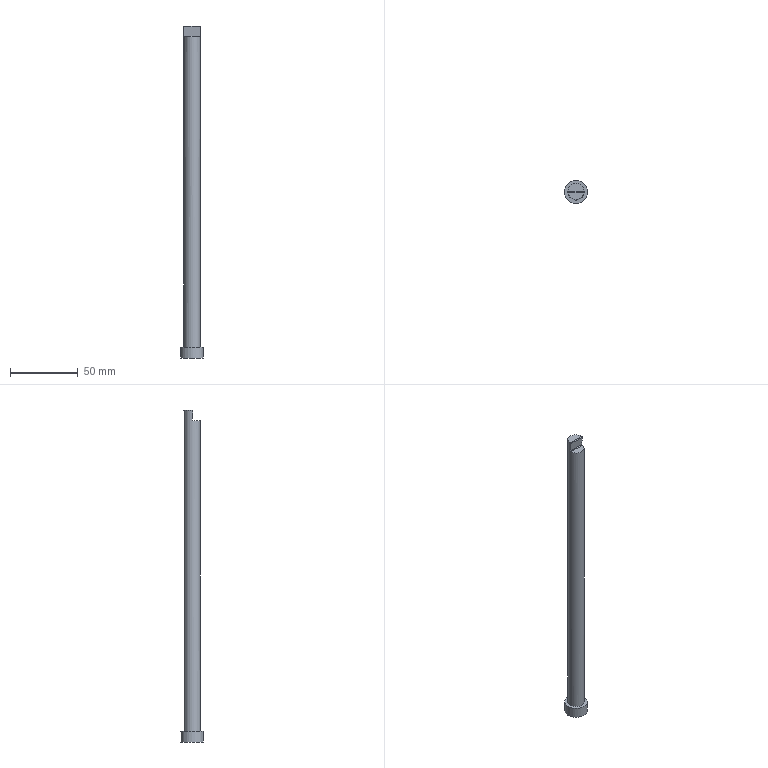Part | NX | features 模具.stp<1>[104] 2 | 1 solid | 9 faces | box 17 x 17 x 245.5 mm | volume 28258 mm3 | plane 5 | cylinder 4 | commonest cylinder face diameters 1 x2 12 x1 17 x1
STEP:
#1=CARTESIAN_POINT('',(-5.998,-0.1543,30.));
#2=VERTEX_POINT('',#1);
#3=CARTESIAN_POINT('',(-5.964,-0.6524,29.456));
#4=VERTEX_POINT('',#3);
#5=CARTESIAN_POINT('',(-5.998,-0.1543,30.));
#6=CARTESIAN_POINT('',(-5.992,-0.406,30.));
#7=CARTESIAN_POINT('',(-5.962,-0.6742,29.706));
#8=CARTESIAN_POINT('',(-5.964,-0.6524,29.456));
#9=B_SPLINE_CURVE_WITH_KNOTS('',3,(#5,#6,#7,#8),.UNSPECIFIED.,.F.,.F.,(4,4),(0.,1.),.UNSPECIFIED.);
#10=EDGE_CURVE('',#2,#4,#9,.T.);
#11=ORIENTED_EDGE('',*,*,#10,.T.);
#12=CARTESIAN_POINT('',(5.964,-0.6524,29.456));
#13=VERTEX_POINT('',#12);
#14=CARTESIAN_POINT('',(6.,-0.6524,29.456));
#15=DIRECTION('',(-1.,0.,0.));
#16=VECTOR('',#15,1000.);
#17=LINE('',#14,#16);
#18=EDGE_CURVE('',#13,#4,#17,.T.);
#19=ORIENTED_EDGE('',*,*,#18,.F.);
#20=CARTESIAN_POINT('',(5.998,-0.1543,30.));
#21=VERTEX_POINT('',#20);
#22=CARTESIAN_POINT('',(5.964,-0.6524,29.456));
#23=CARTESIAN_POINT('',(5.962,-0.6723,29.684));
#24=CARTESIAN_POINT('',(5.99,-0.4503,30.));
#25=CARTESIAN_POINT('',(5.998,-0.1543,30.));
#26=B_SPLINE_CURVE_WITH_KNOTS('',3,(#22,#23,#24,#25),.UNSPECIFIED.,.F.,.F.,(4,4),(0.,1.),.UNSPECIFIED.);
#27=EDGE_CURVE('',#13,#21,#26,.T.);
#28=ORIENTED_EDGE('',*,*,#27,.T.);
#29=CARTESIAN_POINT('',(0.,-0.1543,30.));
#30=DIRECTION('',(-1.,0.,0.));
#31=VECTOR('',#30,1000.);
#32=LINE('',#29,#31);
#33=EDGE_CURVE('',#21,#2,#32,.T.);
#34=ORIENTED_EDGE('',*,*,#33,.T.);
#35=EDGE_LOOP('',(#11,#19,#28,#34));
#36=FACE_BOUND('',#35,.T.);
#37=CARTESIAN_POINT('',(6.,-0.1543,29.5));
#38=DIRECTION('',(1.,0.,0.));
#39=DIRECTION('',(0.,0.,-1.));
#40=AXIS2_PLACEMENT_3D('',#37,#38,#39);
#41=CYLINDRICAL_SURFACE('',#40,0.5);
#42=ADVANCED_FACE('',(#36),#41,.T.);
#43=CARTESIAN_POINT('',(5.975,-0.5457,22.));
#44=VERTEX_POINT('',#43);
#45=CARTESIAN_POINT('',(6.,-0.04756,22.544));
#46=VERTEX_POINT('',#45);
#47=CARTESIAN_POINT('',(5.975,-0.5457,22.));
#48=CARTESIAN_POINT('',(5.987,-0.4152,22.));
#49=CARTESIAN_POINT('',(6.001,-0.1315,22.146));
#50=CARTESIAN_POINT('',(6.,-0.03109,22.355));
#51=CARTESIAN_POINT('',(6.,-0.04756,22.544));
#52=B_SPLINE_CURVE_WITH_KNOTS('',3,(#47,#48,#49,#50,#51),.UNSPECIFIED.,.F.,.F.,(4,1,4),(0.,0.5,1.),.UNSPECIFIED.);
#53=EDGE_CURVE('',#44,#46,#52,.T.);
#54=ORIENTED_EDGE('',*,*,#53,.T.);
#55=CARTESIAN_POINT('',(-6.,-0.04756,22.544));
#56=VERTEX_POINT('',#55);
#57=CARTESIAN_POINT('',(-6.,-0.04756,22.544));
#58=DIRECTION('',(1.,0.,0.));
#59=VECTOR('',#58,1000.);
#60=LINE('',#57,#59);
#61=EDGE_CURVE('',#56,#46,#60,.T.);
#62=ORIENTED_EDGE('',*,*,#61,.F.);
#63=CARTESIAN_POINT('',(-5.975,-0.5457,22.));
#64=VERTEX_POINT('',#63);
#65=CARTESIAN_POINT('',(-6.,-0.04756,22.544));
#66=CARTESIAN_POINT('',(-6.,-0.0311,22.355));
#67=CARTESIAN_POINT('',(-6.001,-0.1312,22.146));
#68=CARTESIAN_POINT('',(-5.987,-0.4151,22.));
#69=CARTESIAN_POINT('',(-5.975,-0.5457,22.));
#70=B_SPLINE_CURVE_WITH_KNOTS('',3,(#65,#66,#67,#68,#69),.UNSPECIFIED.,.F.,.F.,(4,1,4),(0.,0.5,1.),.UNSPECIFIED.);
#71=EDGE_CURVE('',#56,#64,#70,.T.);
#72=ORIENTED_EDGE('',*,*,#71,.T.);
#73=CARTESIAN_POINT('',(6.,-0.5457,22.));
#74=DIRECTION('',(-1.,0.,0.));
#75=VECTOR('',#74,1000.);
#76=LINE('',#73,#75);
#77=EDGE_CURVE('',#44,#64,#76,.T.);
#78=ORIENTED_EDGE('',*,*,#77,.F.);
#79=EDGE_LOOP('',(#54,#62,#72,#78));
#80=FACE_BOUND('',#79,.T.);
#81=CARTESIAN_POINT('',(6.,-0.5457,22.5));
#82=DIRECTION('',(1.,0.,0.));
#83=DIRECTION('',(0.,0.,-1.));
#84=AXIS2_PLACEMENT_3D('',#81,#82,#83);
#85=CYLINDRICAL_SURFACE('',#84,0.5);
#86=ADVANCED_FACE('',(#80),#85,.F.);
#87=CARTESIAN_POINT('',(0.,0.,22.));
#88=DIRECTION('',(0.,0.9962,0.08716));
#89=DIRECTION('',(0.,-0.08716,0.9962));
#90=AXIS2_PLACEMENT_3D('',#87,#88,#89);
#91=ELLIPSE('',#90,68.842,6.);
#92=EDGE_CURVE('',#13,#46,#91,.T.);
#93=ORIENTED_EDGE('',*,*,#92,.F.);
#94=ORIENTED_EDGE('',*,*,#18,.T.);
#95=CARTESIAN_POINT('',(0.,0.,22.));
#96=DIRECTION('',(0.,0.9962,0.08716));
#97=DIRECTION('',(0.,-0.08716,0.9962));
#98=AXIS2_PLACEMENT_3D('',#95,#96,#97);
#99=ELLIPSE('',#98,68.842,6.);
#100=EDGE_CURVE('',#56,#4,#99,.T.);
#101=ORIENTED_EDGE('',*,*,#100,.F.);
#102=ORIENTED_EDGE('',*,*,#61,.T.);
#103=EDGE_LOOP('',(#93,#94,#101,#102));
#104=FACE_BOUND('',#103,.T.);
#105=CARTESIAN_POINT('',(6.,1.046,10.046));
#106=DIRECTION('',(0.,-0.9962,-0.08716));
#107=DIRECTION('',(0.,0.08716,-0.9962));
#108=AXIS2_PLACEMENT_3D('',#105,#106,#107);
#109=PLANE('',#108);
#110=ADVANCED_FACE('',(#104),#109,.T.);
#111=CARTESIAN_POINT('',(0.,0.,22.));
#112=DIRECTION('',(0.,0.,1.));
#113=DIRECTION('',(1.,0.,0.));
#114=AXIS2_PLACEMENT_3D('',#111,#112,#113);
#115=CIRCLE('',#114,6.);
#116=EDGE_CURVE('',#64,#44,#115,.T.);
#117=ORIENTED_EDGE('',*,*,#116,.T.);
#118=ORIENTED_EDGE('',*,*,#77,.T.);
#119=EDGE_LOOP('',(#117,#118));
#120=FACE_BOUND('',#119,.T.);
#121=CARTESIAN_POINT('',(0.,0.,22.));
#122=DIRECTION('',(0.,0.,-1.));
#123=DIRECTION('',(0.,-1.,0.));
#124=AXIS2_PLACEMENT_3D('',#121,#122,#123);
#125=PLANE('',#124);
#126=ADVANCED_FACE('',(#120),#125,.F.);
#127=ORIENTED_EDGE('',*,*,#33,.F.);
#128=CARTESIAN_POINT('',(0.,0.,30.));
#129=DIRECTION('',(0.,0.,-1.));
#130=DIRECTION('',(1.,0.,0.));
#131=AXIS2_PLACEMENT_3D('',#128,#129,#130);
#132=CIRCLE('',#131,6.);
#133=EDGE_CURVE('',#2,#21,#132,.T.);
#134=ORIENTED_EDGE('',*,*,#133,.F.);
#135=EDGE_LOOP('',(#127,#134));
#136=FACE_BOUND('',#135,.T.);
#137=CARTESIAN_POINT('',(0.,0.,30.));
#138=DIRECTION('',(0.,0.,1.));
#139=DIRECTION('',(1.,0.,0.));
#140=AXIS2_PLACEMENT_3D('',#137,#138,#139);
#141=PLANE('',#140);
#142=ADVANCED_FACE('',(#136),#141,.T.);
#143=CARTESIAN_POINT('',(8.5,0.,-215.5));
#144=VERTEX_POINT('',#143);
#145=CARTESIAN_POINT('',(0.,0.,-215.5));
#146=DIRECTION('',(0.,0.,1.));
#147=DIRECTION('',(1.,0.,0.));
#148=AXIS2_PLACEMENT_3D('',#145,#146,#147);
#149=CIRCLE('',#148,8.5);
#150=EDGE_CURVE('',#144,#144,#149,.T.);
#151=ORIENTED_EDGE('',*,*,#150,.T.);
#152=EDGE_LOOP('',(#151));
#153=FACE_BOUND('',#152,.T.);
#154=CARTESIAN_POINT('',(8.5,0.,-207.5));
#155=VERTEX_POINT('',#154);
#156=CARTESIAN_POINT('',(0.,0.,-207.5));
#157=DIRECTION('',(0.,0.,-1.));
#158=DIRECTION('',(1.,0.,0.));
#159=AXIS2_PLACEMENT_3D('',#156,#157,#158);
#160=CIRCLE('',#159,8.5);
#161=EDGE_CURVE('',#155,#155,#160,.T.);
#162=ORIENTED_EDGE('',*,*,#161,.T.);
#163=EDGE_LOOP('',(#162));
#164=FACE_BOUND('',#163,.T.);
#165=CARTESIAN_POINT('',(0.,0.,-215.5));
#166=DIRECTION('',(0.,0.,1.));
#167=DIRECTION('',(1.,0.,0.));
#168=AXIS2_PLACEMENT_3D('',#165,#166,#167);
#169=CYLINDRICAL_SURFACE('',#168,8.5);
#170=ADVANCED_FACE('',(#153,#164),#169,.T.);
#171=ORIENTED_EDGE('',*,*,#150,.F.);
#172=EDGE_LOOP('',(#171));
#173=FACE_BOUND('',#172,.T.);
#174=CARTESIAN_POINT('',(0.,0.,-215.5));
#175=DIRECTION('',(0.,0.,-1.));
#176=DIRECTION('',(0.,-1.,0.));
#177=AXIS2_PLACEMENT_3D('',#174,#175,#176);
#178=PLANE('',#177);
#179=ADVANCED_FACE('',(#173),#178,.T.);
#180=ORIENTED_EDGE('',*,*,#161,.F.);
#181=EDGE_LOOP('',(#180));
#182=FACE_BOUND('',#181,.T.);
#183=CARTESIAN_POINT('',(6.,0.,-207.5));
#184=VERTEX_POINT('',#183);
#185=CARTESIAN_POINT('',(0.,0.,-207.5));
#186=DIRECTION('',(0.,0.,1.));
#187=DIRECTION('',(1.,0.,0.));
#188=AXIS2_PLACEMENT_3D('',#185,#186,#187);
#189=CIRCLE('',#188,6.);
#190=EDGE_CURVE('',#184,#184,#189,.T.);
#191=ORIENTED_EDGE('',*,*,#190,.F.);
#192=EDGE_LOOP('',(#191));
#193=FACE_BOUND('',#192,.T.);
#194=CARTESIAN_POINT('',(0.,0.,-207.5));
#195=DIRECTION('',(0.,0.,1.));
#196=DIRECTION('',(1.,0.,0.));
#197=AXIS2_PLACEMENT_3D('',#194,#195,#196);
#198=PLANE('',#197);
#199=ADVANCED_FACE('',(#182,#193),#198,.T.);
#200=ORIENTED_EDGE('',*,*,#190,.T.);
#201=EDGE_LOOP('',(#200));
#202=FACE_BOUND('',#201,.T.);
#203=ORIENTED_EDGE('',*,*,#10,.F.);
#204=ORIENTED_EDGE('',*,*,#133,.T.);
#205=ORIENTED_EDGE('',*,*,#27,.F.);
#206=ORIENTED_EDGE('',*,*,#92,.T.);
#207=ORIENTED_EDGE('',*,*,#53,.F.);
#208=ORIENTED_EDGE('',*,*,#116,.F.);
#209=ORIENTED_EDGE('',*,*,#71,.F.);
#210=ORIENTED_EDGE('',*,*,#100,.T.);
#211=EDGE_LOOP('',(#203,#204,#205,#206,#207,#208,#209,#210));
#212=FACE_BOUND('',#211,.T.);
#213=CARTESIAN_POINT('',(0.,0.,-215.5));
#214=DIRECTION('',(0.,0.,1.));
#215=DIRECTION('',(1.,0.,0.));
#216=AXIS2_PLACEMENT_3D('',#213,#214,#215);
#217=CYLINDRICAL_SURFACE('',#216,6.);
#218=ADVANCED_FACE('',(#202,#212),#217,.T.);
#219=CLOSED_SHELL('',(#42,#86,#110,#126,#142,#170,#179,#199,#218));
#220=MANIFOLD_SOLID_BREP('',#219);
#221=(LENGTH_UNIT()NAMED_UNIT(*)SI_UNIT(.MILLI.,.METRE.));
#222=UNCERTAINTY_MEASURE_WITH_UNIT(LENGTH_MEASURE(0.0508),#221,'','');
#223=(NAMED_UNIT(*)PLANE_ANGLE_UNIT()SI_UNIT($,.RADIAN.));
#224=(NAMED_UNIT(*)SI_UNIT($,.STERADIAN.)SOLID_ANGLE_UNIT());
#225=(GEOMETRIC_REPRESENTATION_CONTEXT(3)GLOBAL_UNCERTAINTY_ASSIGNED_CONTEXT((#222))GLOBAL_UNIT_ASSIGNED_CONTEXT((#221,#223,#224))REPRESENTATION_CONTEXT('',''));
#226=ADVANCED_BREP_SHAPE_REPRESENTATION('',(#220),#225);